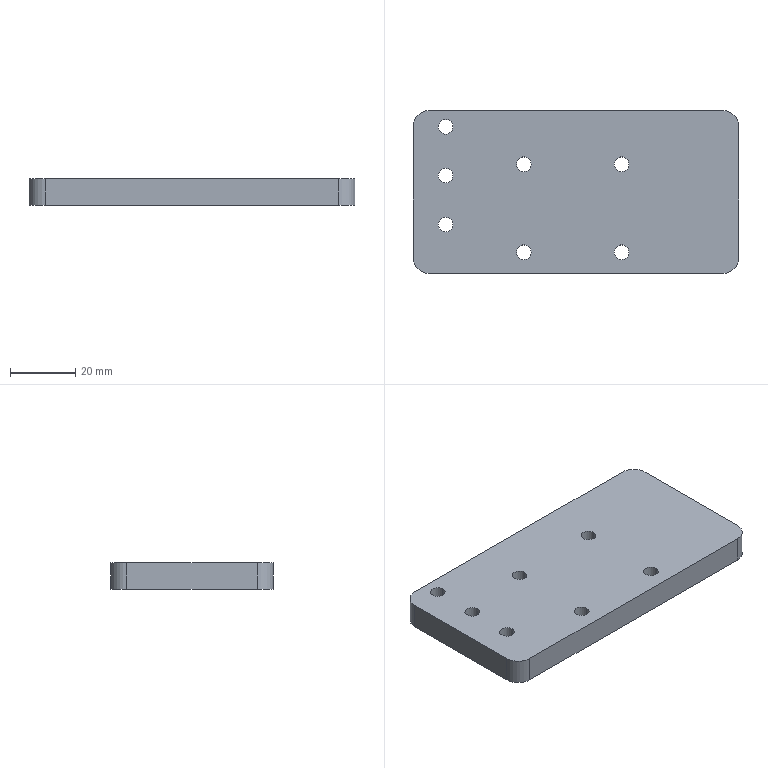Part | STEP file | 08-23 side baffle fixing plate A | 1 solid | 45 faces | box 100 x 50 x 8 mm | volume 37879 mm3 | cylinder 32 | plane 13 | commonest cylinder face diameters 4.5 x14 8 x14 10 x4
STEP:
#1=CARTESIAN_POINT('',(-36.,20.,4.4));
#2=VERTEX_POINT('',#1);
#3=CARTESIAN_POINT('',(-44.,20.,4.4));
#4=VERTEX_POINT('',#3);
#5=CARTESIAN_POINT('',(-40.,20.,4.4));
#6=DIRECTION('',(0.,0.,-1.));
#7=DIRECTION('',(-1.,0.,0.));
#8=AXIS2_PLACEMENT_3D('',#5,#6,#7);
#9=CIRCLE('',#8,4.);
#10=EDGE_CURVE('',#2,#4,#9,.T.);
#11=ORIENTED_EDGE('',*,*,#10,.F.);
#12=CARTESIAN_POINT('',(-36.,20.,0.));
#13=VERTEX_POINT('',#12);
#14=CARTESIAN_POINT('',(-36.,20.,0.));
#15=DIRECTION('',(0.,0.,-1.));
#16=VECTOR('',#15,1000.);
#17=LINE('',#14,#16);
#18=EDGE_CURVE('',#2,#13,#17,.T.);
#19=ORIENTED_EDGE('',*,*,#18,.T.);
#20=CARTESIAN_POINT('',(-44.,20.,0.));
#21=VERTEX_POINT('',#20);
#22=CARTESIAN_POINT('',(-40.,20.,0.));
#23=DIRECTION('',(0.,0.,-1.));
#24=DIRECTION('',(-1.,0.,0.));
#25=AXIS2_PLACEMENT_3D('',#22,#23,#24);
#26=CIRCLE('',#25,4.);
#27=EDGE_CURVE('',#13,#21,#26,.T.);
#28=ORIENTED_EDGE('',*,*,#27,.T.);
#29=CARTESIAN_POINT('',(-44.,20.,0.));
#30=DIRECTION('',(0.,0.,-1.));
#31=VECTOR('',#30,1000.);
#32=LINE('',#29,#31);
#33=EDGE_CURVE('',#4,#21,#32,.T.);
#34=ORIENTED_EDGE('',*,*,#33,.F.);
#35=EDGE_LOOP('',(#11,#19,#28,#34));
#36=FACE_OUTER_BOUND('',#35,.T.);
#37=CARTESIAN_POINT('',(-40.,20.,0.));
#38=DIRECTION('',(0.,0.,-1.));
#39=DIRECTION('',(-1.,0.,0.));
#40=AXIS2_PLACEMENT_3D('',#37,#38,#39);
#41=CYLINDRICAL_SURFACE('',#40,4.);
#42=ADVANCED_FACE('',(#36),#41,.F.);
#43=CARTESIAN_POINT('',(-37.75,20.,8.));
#44=VERTEX_POINT('',#43);
#45=CARTESIAN_POINT('',(-42.25,20.,8.));
#46=VERTEX_POINT('',#45);
#47=CARTESIAN_POINT('',(-40.,20.,8.));
#48=DIRECTION('',(0.,0.,-1.));
#49=DIRECTION('',(-1.,0.,0.));
#50=AXIS2_PLACEMENT_3D('',#47,#48,#49);
#51=CIRCLE('',#50,2.25);
#52=EDGE_CURVE('',#44,#46,#51,.T.);
#53=ORIENTED_EDGE('',*,*,#52,.F.);
#54=CARTESIAN_POINT('',(-37.75,20.,4.4));
#55=VERTEX_POINT('',#54);
#56=CARTESIAN_POINT('',(-37.75,20.,0.));
#57=DIRECTION('',(0.,0.,-1.));
#58=VECTOR('',#57,1000.);
#59=LINE('',#56,#58);
#60=EDGE_CURVE('',#44,#55,#59,.T.);
#61=ORIENTED_EDGE('',*,*,#60,.T.);
#62=CARTESIAN_POINT('',(-42.25,20.,4.4));
#63=VERTEX_POINT('',#62);
#64=CARTESIAN_POINT('',(-40.,20.,4.4));
#65=DIRECTION('',(0.,0.,-1.));
#66=DIRECTION('',(-1.,0.,0.));
#67=AXIS2_PLACEMENT_3D('',#64,#65,#66);
#68=CIRCLE('',#67,2.25);
#69=EDGE_CURVE('',#55,#63,#68,.T.);
#70=ORIENTED_EDGE('',*,*,#69,.T.);
#71=CARTESIAN_POINT('',(-42.25,20.,0.));
#72=DIRECTION('',(0.,0.,-1.));
#73=VECTOR('',#72,1000.);
#74=LINE('',#71,#73);
#75=EDGE_CURVE('',#46,#63,#74,.T.);
#76=ORIENTED_EDGE('',*,*,#75,.F.);
#77=EDGE_LOOP('',(#53,#61,#70,#76));
#78=FACE_OUTER_BOUND('',#77,.T.);
#79=CARTESIAN_POINT('',(-40.,20.,0.));
#80=DIRECTION('',(0.,0.,-1.));
#81=DIRECTION('',(-1.,0.,0.));
#82=AXIS2_PLACEMENT_3D('',#79,#80,#81);
#83=CYLINDRICAL_SURFACE('',#82,2.25);
#84=ADVANCED_FACE('',(#78),#83,.F.);
#85=CARTESIAN_POINT('',(-36.,5.,4.4));
#86=VERTEX_POINT('',#85);
#87=CARTESIAN_POINT('',(-44.,5.,4.4));
#88=VERTEX_POINT('',#87);
#89=CARTESIAN_POINT('',(-40.,5.,4.4));
#90=DIRECTION('',(0.,0.,-1.));
#91=DIRECTION('',(-1.,0.,0.));
#92=AXIS2_PLACEMENT_3D('',#89,#90,#91);
#93=CIRCLE('',#92,4.);
#94=EDGE_CURVE('',#86,#88,#93,.T.);
#95=ORIENTED_EDGE('',*,*,#94,.F.);
#96=CARTESIAN_POINT('',(-36.,5.,0.));
#97=VERTEX_POINT('',#96);
#98=CARTESIAN_POINT('',(-36.,5.,0.));
#99=DIRECTION('',(0.,0.,-1.));
#100=VECTOR('',#99,1000.);
#101=LINE('',#98,#100);
#102=EDGE_CURVE('',#86,#97,#101,.T.);
#103=ORIENTED_EDGE('',*,*,#102,.T.);
#104=CARTESIAN_POINT('',(-44.,5.,0.));
#105=VERTEX_POINT('',#104);
#106=CARTESIAN_POINT('',(-40.,5.,0.));
#107=DIRECTION('',(0.,0.,-1.));
#108=DIRECTION('',(-1.,0.,0.));
#109=AXIS2_PLACEMENT_3D('',#106,#107,#108);
#110=CIRCLE('',#109,4.);
#111=EDGE_CURVE('',#97,#105,#110,.T.);
#112=ORIENTED_EDGE('',*,*,#111,.T.);
#113=CARTESIAN_POINT('',(-44.,5.,0.));
#114=DIRECTION('',(0.,0.,-1.));
#115=VECTOR('',#114,1000.);
#116=LINE('',#113,#115);
#117=EDGE_CURVE('',#88,#105,#116,.T.);
#118=ORIENTED_EDGE('',*,*,#117,.F.);
#119=EDGE_LOOP('',(#95,#103,#112,#118));
#120=FACE_OUTER_BOUND('',#119,.T.);
#121=CARTESIAN_POINT('',(-40.,5.,0.));
#122=DIRECTION('',(0.,0.,-1.));
#123=DIRECTION('',(-1.,0.,0.));
#124=AXIS2_PLACEMENT_3D('',#121,#122,#123);
#125=CYLINDRICAL_SURFACE('',#124,4.);
#126=ADVANCED_FACE('',(#120),#125,.F.);
#127=CARTESIAN_POINT('',(-37.75,5.,8.));
#128=VERTEX_POINT('',#127);
#129=CARTESIAN_POINT('',(-42.25,5.,8.));
#130=VERTEX_POINT('',#129);
#131=CARTESIAN_POINT('',(-40.,5.,8.));
#132=DIRECTION('',(0.,0.,-1.));
#133=DIRECTION('',(-1.,0.,0.));
#134=AXIS2_PLACEMENT_3D('',#131,#132,#133);
#135=CIRCLE('',#134,2.25);
#136=EDGE_CURVE('',#128,#130,#135,.T.);
#137=ORIENTED_EDGE('',*,*,#136,.F.);
#138=CARTESIAN_POINT('',(-37.75,5.,4.4));
#139=VERTEX_POINT('',#138);
#140=CARTESIAN_POINT('',(-37.75,5.,0.));
#141=DIRECTION('',(0.,0.,-1.));
#142=VECTOR('',#141,1000.);
#143=LINE('',#140,#142);
#144=EDGE_CURVE('',#128,#139,#143,.T.);
#145=ORIENTED_EDGE('',*,*,#144,.T.);
#146=CARTESIAN_POINT('',(-42.25,5.,4.4));
#147=VERTEX_POINT('',#146);
#148=CARTESIAN_POINT('',(-40.,5.,4.4));
#149=DIRECTION('',(0.,0.,-1.));
#150=DIRECTION('',(-1.,0.,0.));
#151=AXIS2_PLACEMENT_3D('',#148,#149,#150);
#152=CIRCLE('',#151,2.25);
#153=EDGE_CURVE('',#139,#147,#152,.T.);
#154=ORIENTED_EDGE('',*,*,#153,.T.);
#155=CARTESIAN_POINT('',(-42.25,5.,0.));
#156=DIRECTION('',(0.,0.,-1.));
#157=VECTOR('',#156,1000.);
#158=LINE('',#155,#157);
#159=EDGE_CURVE('',#130,#147,#158,.T.);
#160=ORIENTED_EDGE('',*,*,#159,.F.);
#161=EDGE_LOOP('',(#137,#145,#154,#160));
#162=FACE_OUTER_BOUND('',#161,.T.);
#163=CARTESIAN_POINT('',(-40.,5.,0.));
#164=DIRECTION('',(0.,0.,-1.));
#165=DIRECTION('',(-1.,0.,0.));
#166=AXIS2_PLACEMENT_3D('',#163,#164,#165);
#167=CYLINDRICAL_SURFACE('',#166,2.25);
#168=ADVANCED_FACE('',(#162),#167,.F.);
#169=CARTESIAN_POINT('',(-36.,-10.,4.4));
#170=VERTEX_POINT('',#169);
#171=CARTESIAN_POINT('',(-44.,-10.,4.4));
#172=VERTEX_POINT('',#171);
#173=CARTESIAN_POINT('',(-40.,-10.,4.4));
#174=DIRECTION('',(0.,0.,-1.));
#175=DIRECTION('',(-1.,0.,0.));
#176=AXIS2_PLACEMENT_3D('',#173,#174,#175);
#177=CIRCLE('',#176,4.);
#178=EDGE_CURVE('',#170,#172,#177,.T.);
#179=ORIENTED_EDGE('',*,*,#178,.F.);
#180=CARTESIAN_POINT('',(-36.,-10.,0.));
#181=VERTEX_POINT('',#180);
#182=CARTESIAN_POINT('',(-36.,-10.,0.));
#183=DIRECTION('',(0.,0.,-1.));
#184=VECTOR('',#183,1000.);
#185=LINE('',#182,#184);
#186=EDGE_CURVE('',#170,#181,#185,.T.);
#187=ORIENTED_EDGE('',*,*,#186,.T.);
#188=CARTESIAN_POINT('',(-44.,-10.,0.));
#189=VERTEX_POINT('',#188);
#190=CARTESIAN_POINT('',(-40.,-10.,0.));
#191=DIRECTION('',(0.,0.,-1.));
#192=DIRECTION('',(-1.,0.,0.));
#193=AXIS2_PLACEMENT_3D('',#190,#191,#192);
#194=CIRCLE('',#193,4.);
#195=EDGE_CURVE('',#181,#189,#194,.T.);
#196=ORIENTED_EDGE('',*,*,#195,.T.);
#197=CARTESIAN_POINT('',(-44.,-10.,0.));
#198=DIRECTION('',(0.,0.,-1.));
#199=VECTOR('',#198,1000.);
#200=LINE('',#197,#199);
#201=EDGE_CURVE('',#172,#189,#200,.T.);
#202=ORIENTED_EDGE('',*,*,#201,.F.);
#203=EDGE_LOOP('',(#179,#187,#196,#202));
#204=FACE_OUTER_BOUND('',#203,.T.);
#205=CARTESIAN_POINT('',(-40.,-10.,0.));
#206=DIRECTION('',(0.,0.,-1.));
#207=DIRECTION('',(-1.,0.,0.));
#208=AXIS2_PLACEMENT_3D('',#205,#206,#207);
#209=CYLINDRICAL_SURFACE('',#208,4.);
#210=ADVANCED_FACE('',(#204),#209,.F.);
#211=CARTESIAN_POINT('',(-37.75,-10.,8.));
#212=VERTEX_POINT('',#211);
#213=CARTESIAN_POINT('',(-42.25,-10.,8.));
#214=VERTEX_POINT('',#213);
#215=CARTESIAN_POINT('',(-40.,-10.,8.));
#216=DIRECTION('',(0.,0.,-1.));
#217=DIRECTION('',(-1.,0.,0.));
#218=AXIS2_PLACEMENT_3D('',#215,#216,#217);
#219=CIRCLE('',#218,2.25);
#220=EDGE_CURVE('',#212,#214,#219,.T.);
#221=ORIENTED_EDGE('',*,*,#220,.F.);
#222=CARTESIAN_POINT('',(-37.75,-10.,4.4));
#223=VERTEX_POINT('',#222);
#224=CARTESIAN_POINT('',(-37.75,-10.,0.));
#225=DIRECTION('',(0.,0.,-1.));
#226=VECTOR('',#225,1000.);
#227=LINE('',#224,#226);
#228=EDGE_CURVE('',#212,#223,#227,.T.);
#229=ORIENTED_EDGE('',*,*,#228,.T.);
#230=CARTESIAN_POINT('',(-42.25,-10.,4.4));
#231=VERTEX_POINT('',#230);
#232=CARTESIAN_POINT('',(-40.,-10.,4.4));
#233=DIRECTION('',(0.,0.,-1.));
#234=DIRECTION('',(-1.,0.,0.));
#235=AXIS2_PLACEMENT_3D('',#232,#233,#234);
#236=CIRCLE('',#235,2.25);
#237=EDGE_CURVE('',#223,#231,#236,.T.);
#238=ORIENTED_EDGE('',*,*,#237,.T.);
#239=CARTESIAN_POINT('',(-42.25,-10.,0.));
#240=DIRECTION('',(0.,0.,-1.));
#241=VECTOR('',#240,1000.);
#242=LINE('',#239,#241);
#243=EDGE_CURVE('',#214,#231,#242,.T.);
#244=ORIENTED_EDGE('',*,*,#243,.F.);
#245=EDGE_LOOP('',(#221,#229,#238,#244));
#246=FACE_OUTER_BOUND('',#245,.T.);
#247=CARTESIAN_POINT('',(-40.,-10.,0.));
#248=DIRECTION('',(0.,0.,-1.));
#249=DIRECTION('',(-1.,0.,0.));
#250=AXIS2_PLACEMENT_3D('',#247,#248,#249);
#251=CYLINDRICAL_SURFACE('',#250,2.25);
#252=ADVANCED_FACE('',(#246),#251,.F.);
#253=CARTESIAN_POINT('',(18.,8.5,4.4));
#254=VERTEX_POINT('',#253);
#255=CARTESIAN_POINT('',(10.,8.5,4.4));
#256=VERTEX_POINT('',#255);
#257=CARTESIAN_POINT('',(14.,8.5,4.4));
#258=DIRECTION('',(0.,0.,-1.));
#259=DIRECTION('',(-1.,0.,0.));
#260=AXIS2_PLACEMENT_3D('',#257,#258,#259);
#261=CIRCLE('',#260,4.);
#262=EDGE_CURVE('',#254,#256,#261,.T.);
#263=ORIENTED_EDGE('',*,*,#262,.F.);
#264=CARTESIAN_POINT('',(18.,8.5,0.));
#265=VERTEX_POINT('',#264);
#266=CARTESIAN_POINT('',(18.,8.5,0.));
#267=DIRECTION('',(0.,0.,-1.));
#268=VECTOR('',#267,1000.);
#269=LINE('',#266,#268);
#270=EDGE_CURVE('',#254,#265,#269,.T.);
#271=ORIENTED_EDGE('',*,*,#270,.T.);
#272=CARTESIAN_POINT('',(10.,8.5,0.));
#273=VERTEX_POINT('',#272);
#274=CARTESIAN_POINT('',(14.,8.5,0.));
#275=DIRECTION('',(0.,0.,-1.));
#276=DIRECTION('',(-1.,0.,0.));
#277=AXIS2_PLACEMENT_3D('',#274,#275,#276);
#278=CIRCLE('',#277,4.);
#279=EDGE_CURVE('',#265,#273,#278,.T.);
#280=ORIENTED_EDGE('',*,*,#279,.T.);
#281=CARTESIAN_POINT('',(10.,8.5,0.));
#282=DIRECTION('',(0.,0.,-1.));
#283=VECTOR('',#282,1000.);
#284=LINE('',#281,#283);
#285=EDGE_CURVE('',#256,#273,#284,.T.);
#286=ORIENTED_EDGE('',*,*,#285,.F.);
#287=EDGE_LOOP('',(#263,#271,#280,#286));
#288=FACE_OUTER_BOUND('',#287,.T.);
#289=CARTESIAN_POINT('',(14.,8.5,0.));
#290=DIRECTION('',(0.,0.,-1.));
#291=DIRECTION('',(-1.,0.,0.));
#292=AXIS2_PLACEMENT_3D('',#289,#290,#291);
#293=CYLINDRICAL_SURFACE('',#292,4.);
#294=ADVANCED_FACE('',(#288),#293,.F.);
#295=CARTESIAN_POINT('',(16.25,8.5,8.));
#296=VERTEX_POINT('',#295);
#297=CARTESIAN_POINT('',(11.75,8.5,8.));
#298=VERTEX_POINT('',#297);
#299=CARTESIAN_POINT('',(14.,8.5,8.));
#300=DIRECTION('',(0.,0.,-1.));
#301=DIRECTION('',(-1.,0.,0.));
#302=AXIS2_PLACEMENT_3D('',#299,#300,#301);
#303=CIRCLE('',#302,2.25);
#304=EDGE_CURVE('',#296,#298,#303,.T.);
#305=ORIENTED_EDGE('',*,*,#304,.F.);
#306=CARTESIAN_POINT('',(16.25,8.5,4.4));
#307=VERTEX_POINT('',#306);
#308=CARTESIAN_POINT('',(16.25,8.5,0.));
#309=DIRECTION('',(0.,0.,-1.));
#310=VECTOR('',#309,1000.);
#311=LINE('',#308,#310);
#312=EDGE_CURVE('',#296,#307,#311,.T.);
#313=ORIENTED_EDGE('',*,*,#312,.T.);
#314=CARTESIAN_POINT('',(11.75,8.5,4.4));
#315=VERTEX_POINT('',#314);
#316=CARTESIAN_POINT('',(14.,8.5,4.4));
#317=DIRECTION('',(0.,0.,-1.));
#318=DIRECTION('',(-1.,0.,0.));
#319=AXIS2_PLACEMENT_3D('',#316,#317,#318);
#320=CIRCLE('',#319,2.25);
#321=EDGE_CURVE('',#307,#315,#320,.T.);
#322=ORIENTED_EDGE('',*,*,#321,.T.);
#323=CARTESIAN_POINT('',(11.75,8.5,0.));
#324=DIRECTION('',(0.,0.,-1.));
#325=VECTOR('',#324,1000.);
#326=LINE('',#323,#325);
#327=EDGE_CURVE('',#298,#315,#326,.T.);
#328=ORIENTED_EDGE('',*,*,#327,.F.);
#329=EDGE_LOOP('',(#305,#313,#322,#328));
#330=FACE_OUTER_BOUND('',#329,.T.);
#331=CARTESIAN_POINT('',(14.,8.5,0.));
#332=DIRECTION('',(0.,0.,-1.));
#333=DIRECTION('',(-1.,0.,0.));
#334=AXIS2_PLACEMENT_3D('',#331,#332,#333);
#335=CYLINDRICAL_SURFACE('',#334,2.25);
#336=ADVANCED_FACE('',(#330),#335,.F.);
#337=CARTESIAN_POINT('',(-12.,8.5,4.4));
#338=VERTEX_POINT('',#337);
#339=CARTESIAN_POINT('',(-20.,8.5,4.4));
#340=VERTEX_POINT('',#339);
#341=CARTESIAN_POINT('',(-16.,8.5,4.4));
#342=DIRECTION('',(0.,0.,-1.));
#343=DIRECTION('',(-1.,0.,0.));
#344=AXIS2_PLACEMENT_3D('',#341,#342,#343);
#345=CIRCLE('',#344,4.);
#346=EDGE_CURVE('',#338,#340,#345,.T.);
#347=ORIENTED_EDGE('',*,*,#346,.F.);
#348=CARTESIAN_POINT('',(-12.,8.5,0.));
#349=VERTEX_POINT('',#348);
#350=CARTESIAN_POINT('',(-12.,8.5,0.));
#351=DIRECTION('',(0.,0.,-1.));
#352=VECTOR('',#351,1000.);
#353=LINE('',#350,#352);
#354=EDGE_CURVE('',#338,#349,#353,.T.);
#355=ORIENTED_EDGE('',*,*,#354,.T.);
#356=CARTESIAN_POINT('',(-20.,8.5,0.));
#357=VERTEX_POINT('',#356);
#358=CARTESIAN_POINT('',(-16.,8.5,0.));
#359=DIRECTION('',(0.,0.,-1.));
#360=DIRECTION('',(-1.,0.,0.));
#361=AXIS2_PLACEMENT_3D('',#358,#359,#360);
#362=CIRCLE('',#361,4.);
#363=EDGE_CURVE('',#349,#357,#362,.T.);
#364=ORIENTED_EDGE('',*,*,#363,.T.);
#365=CARTESIAN_POINT('',(-20.,8.5,0.));
#366=DIRECTION('',(0.,0.,-1.));
#367=VECTOR('',#366,1000.);
#368=LINE('',#365,#367);
#369=EDGE_CURVE('',#340,#357,#368,.T.);
#370=ORIENTED_EDGE('',*,*,#369,.F.);
#371=EDGE_LOOP('',(#347,#355,#364,#370));
#372=FACE_OUTER_BOUND('',#371,.T.);
#373=CARTESIAN_POINT('',(-16.,8.5,0.));
#374=DIRECTION('',(0.,0.,-1.));
#375=DIRECTION('',(-1.,0.,0.));
#376=AXIS2_PLACEMENT_3D('',#373,#374,#375);
#377=CYLINDRICAL_SURFACE('',#376,4.);
#378=ADVANCED_FACE('',(#372),#377,.F.);
#379=CARTESIAN_POINT('',(-13.75,8.5,8.));
#380=VERTEX_POINT('',#379);
#381=CARTESIAN_POINT('',(-18.25,8.5,8.));
#382=VERTEX_POINT('',#381);
#383=CARTESIAN_POINT('',(-16.,8.5,8.));
#384=DIRECTION('',(0.,0.,-1.));
#385=DIRECTION('',(-1.,0.,0.));
#386=AXIS2_PLACEMENT_3D('',#383,#384,#385);
#387=CIRCLE('',#386,2.25);
#388=EDGE_CURVE('',#380,#382,#387,.T.);
#389=ORIENTED_EDGE('',*,*,#388,.F.);
#390=CARTESIAN_POINT('',(-13.75,8.5,4.4));
#391=VERTEX_POINT('',#390);
#392=CARTESIAN_POINT('',(-13.75,8.5,0.));
#393=DIRECTION('',(0.,0.,-1.));
#394=VECTOR('',#393,1000.);
#395=LINE('',#392,#394);
#396=EDGE_CURVE('',#380,#391,#395,.T.);
#397=ORIENTED_EDGE('',*,*,#396,.T.);
#398=CARTESIAN_POINT('',(-18.25,8.5,4.4));
#399=VERTEX_POINT('',#398);
#400=CARTESIAN_POINT('',(-16.,8.5,4.4));
#401=DIRECTION('',(0.,0.,-1.));
#402=DIRECTION('',(-1.,0.,0.));
#403=AXIS2_PLACEMENT_3D('',#400,#401,#402);
#404=CIRCLE('',#403,2.25);
#405=EDGE_CURVE('',#391,#399,#404,.T.);
#406=ORIENTED_EDGE('',*,*,#405,.T.);
#407=CARTESIAN_POINT('',(-18.25,8.5,0.));
#408=DIRECTION('',(0.,0.,-1.));
#409=VECTOR('',#408,1000.);
#410=LINE('',#407,#409);
#411=EDGE_CURVE('',#382,#399,#410,.T.);
#412=ORIENTED_EDGE('',*,*,#411,.F.);
#413=EDGE_LOOP('',(#389,#397,#406,#412));
#414=FACE_OUTER_BOUND('',#413,.T.);
#415=CARTESIAN_POINT('',(-16.,8.5,0.));
#416=DIRECTION('',(0.,0.,-1.));
#417=DIRECTION('',(-1.,0.,0.));
#418=AXIS2_PLACEMENT_3D('',#415,#416,#417);
#419=CYLINDRICAL_SURFACE('',#418,2.25);
#420=ADVANCED_FACE('',(#414),#419,.F.);
#421=CARTESIAN_POINT('',(-12.,-18.5,4.4));
#422=VERTEX_POINT('',#421);
#423=CARTESIAN_POINT('',(-20.,-18.5,4.4));
#424=VERTEX_POINT('',#423);
#425=CARTESIAN_POINT('',(-16.,-18.5,4.4));
#426=DIRECTION('',(0.,0.,-1.));
#427=DIRECTION('',(-1.,0.,0.));
#428=AXIS2_PLACEMENT_3D('',#425,#426,#427);
#429=CIRCLE('',#428,4.);
#430=EDGE_CURVE('',#422,#424,#429,.T.);
#431=ORIENTED_EDGE('',*,*,#430,.F.);
#432=CARTESIAN_POINT('',(-12.,-18.5,0.));
#433=VERTEX_POINT('',#432);
#434=CARTESIAN_POINT('',(-12.,-18.5,0.));
#435=DIRECTION('',(0.,0.,-1.));
#436=VECTOR('',#435,1000.);
#437=LINE('',#434,#436);
#438=EDGE_CURVE('',#422,#433,#437,.T.);
#439=ORIENTED_EDGE('',*,*,#438,.T.);
#440=CARTESIAN_POINT('',(-20.,-18.5,0.));
#441=VERTEX_POINT('',#440);
#442=CARTESIAN_POINT('',(-16.,-18.5,0.));
#443=DIRECTION('',(0.,0.,-1.));
#444=DIRECTION('',(-1.,0.,0.));
#445=AXIS2_PLACEMENT_3D('',#442,#443,#444);
#446=CIRCLE('',#445,4.);
#447=EDGE_CURVE('',#433,#441,#446,.T.);
#448=ORIENTED_EDGE('',*,*,#447,.T.);
#449=CARTESIAN_POINT('',(-20.,-18.5,0.));
#450=DIRECTION('',(0.,0.,-1.));
#451=VECTOR('',#450,1000.);
#452=LINE('',#449,#451);
#453=EDGE_CURVE('',#424,#441,#452,.T.);
#454=ORIENTED_EDGE('',*,*,#453,.F.);
#455=EDGE_LOOP('',(#431,#439,#448,#454));
#456=FACE_OUTER_BOUND('',#455,.T.);
#457=CARTESIAN_POINT('',(-16.,-18.5,0.));
#458=DIRECTION('',(0.,0.,-1.));
#459=DIRECTION('',(-1.,0.,0.));
#460=AXIS2_PLACEMENT_3D('',#457,#458,#459);
#461=CYLINDRICAL_SURFACE('',#460,4.);
#462=ADVANCED_FACE('',(#456),#461,.F.);
#463=CARTESIAN_POINT('',(-13.75,-18.5,8.));
#464=VERTEX_POINT('',#463);
#465=CARTESIAN_POINT('',(-18.25,-18.5,8.));
#466=VERTEX_POINT('',#465);
#467=CARTESIAN_POINT('',(-16.,-18.5,8.));
#468=DIRECTION('',(0.,0.,-1.));
#469=DIRECTION('',(-1.,0.,0.));
#470=AXIS2_PLACEMENT_3D('',#467,#468,#469);
#471=CIRCLE('',#470,2.25);
#472=EDGE_CURVE('',#464,#466,#471,.T.);
#473=ORIENTED_EDGE('',*,*,#472,.F.);
#474=CARTESIAN_POINT('',(-13.75,-18.5,4.4));
#475=VERTEX_POINT('',#474);
#476=CARTESIAN_POINT('',(-13.75,-18.5,0.));
#477=DIRECTION('',(0.,0.,-1.));
#478=VECTOR('',#477,1000.);
#479=LINE('',#476,#478);
#480=EDGE_CURVE('',#464,#475,#479,.T.);
#481=ORIENTED_EDGE('',*,*,#480,.T.);
#482=CARTESIAN_POINT('',(-18.25,-18.5,4.4));
#483=VERTEX_POINT('',#482);
#484=CARTESIAN_POINT('',(-16.,-18.5,4.4));
#485=DIRECTION('',(0.,0.,-1.));
#486=DIRECTION('',(-1.,0.,0.));
#487=AXIS2_PLACEMENT_3D('',#484,#485,#486);
#488=CIRCLE('',#487,2.25);
#489=EDGE_CURVE('',#475,#483,#488,.T.);
#490=ORIENTED_EDGE('',*,*,#489,.T.);
#491=CARTESIAN_POINT('',(-18.25,-18.5,0.));
#492=DIRECTION('',(0.,0.,-1.));
#493=VECTOR('',#492,1000.);
#494=LINE('',#491,#493);
#495=EDGE_CURVE('',#466,#483,#494,.T.);
#496=ORIENTED_EDGE('',*,*,#495,.F.);
#497=EDGE_LOOP('',(#473,#481,#490,#496));
#498=FACE_OUTER_BOUND('',#497,.T.);
#499=CARTESIAN_POINT('',(-16.,-18.5,0.));
#500=DIRECTION('',(0.,0.,-1.));
#501=DIRECTION('',(-1.,0.,0.));
#502=AXIS2_PLACEMENT_3D('',#499,#500,#501);
#503=CYLINDRICAL_SURFACE('',#502,2.25);
#504=ADVANCED_FACE('',(#498),#503,.F.);
#505=CARTESIAN_POINT('',(18.,-18.5,4.4));
#506=VERTEX_POINT('',#505);
#507=CARTESIAN_POINT('',(10.,-18.5,4.4));
#508=VERTEX_POINT('',#507);
#509=CARTESIAN_POINT('',(14.,-18.5,4.4));
#510=DIRECTION('',(0.,0.,-1.));
#511=DIRECTION('',(-1.,0.,0.));
#512=AXIS2_PLACEMENT_3D('',#509,#510,#511);
#513=CIRCLE('',#512,4.);
#514=EDGE_CURVE('',#506,#508,#513,.T.);
#515=ORIENTED_EDGE('',*,*,#514,.F.);
#516=CARTESIAN_POINT('',(18.,-18.5,0.));
#517=VERTEX_POINT('',#516);
#518=CARTESIAN_POINT('',(18.,-18.5,0.));
#519=DIRECTION('',(0.,0.,-1.));
#520=VECTOR('',#519,1000.);
#521=LINE('',#518,#520);
#522=EDGE_CURVE('',#506,#517,#521,.T.);
#523=ORIENTED_EDGE('',*,*,#522,.T.);
#524=CARTESIAN_POINT('',(10.,-18.5,0.));
#525=VERTEX_POINT('',#524);
#526=CARTESIAN_POINT('',(14.,-18.5,0.));
#527=DIRECTION('',(0.,0.,-1.));
#528=DIRECTION('',(-1.,0.,0.));
#529=AXIS2_PLACEMENT_3D('',#526,#527,#528);
#530=CIRCLE('',#529,4.);
#531=EDGE_CURVE('',#517,#525,#530,.T.);
#532=ORIENTED_EDGE('',*,*,#531,.T.);
#533=CARTESIAN_POINT('',(10.,-18.5,0.));
#534=DIRECTION('',(0.,0.,-1.));
#535=VECTOR('',#534,1000.);
#536=LINE('',#533,#535);
#537=EDGE_CURVE('',#508,#525,#536,.T.);
#538=ORIENTED_EDGE('',*,*,#537,.F.);
#539=EDGE_LOOP('',(#515,#523,#532,#538));
#540=FACE_OUTER_BOUND('',#539,.T.);
#541=CARTESIAN_POINT('',(14.,-18.5,0.));
#542=DIRECTION('',(0.,0.,-1.));
#543=DIRECTION('',(-1.,0.,0.));
#544=AXIS2_PLACEMENT_3D('',#541,#542,#543);
#545=CYLINDRICAL_SURFACE('',#544,4.);
#546=ADVANCED_FACE('',(#540),#545,.F.);
#547=CARTESIAN_POINT('',(16.25,-18.5,8.));
#548=VERTEX_POINT('',#547);
#549=CARTESIAN_POINT('',(11.75,-18.5,8.));
#550=VERTEX_POINT('',#549);
#551=CARTESIAN_POINT('',(14.,-18.5,8.));
#552=DIRECTION('',(0.,0.,-1.));
#553=DIRECTION('',(-1.,0.,0.));
#554=AXIS2_PLACEMENT_3D('',#551,#552,#553);
#555=CIRCLE('',#554,2.25);
#556=EDGE_CURVE('',#548,#550,#555,.T.);
#557=ORIENTED_EDGE('',*,*,#556,.F.);
#558=CARTESIAN_POINT('',(16.25,-18.5,4.4));
#559=VERTEX_POINT('',#558);
#560=CARTESIAN_POINT('',(16.25,-18.5,0.));
#561=DIRECTION('',(0.,0.,-1.));
#562=VECTOR('',#561,1000.);
#563=LINE('',#560,#562);
#564=EDGE_CURVE('',#548,#559,#563,.T.);
#565=ORIENTED_EDGE('',*,*,#564,.T.);
#566=CARTESIAN_POINT('',(11.75,-18.5,4.4));
#567=VERTEX_POINT('',#566);
#568=CARTESIAN_POINT('',(14.,-18.5,4.4));
#569=DIRECTION('',(0.,0.,-1.));
#570=DIRECTION('',(-1.,0.,0.));
#571=AXIS2_PLACEMENT_3D('',#568,#569,#570);
#572=CIRCLE('',#571,2.25);
#573=EDGE_CURVE('',#559,#567,#572,.T.);
#574=ORIENTED_EDGE('',*,*,#573,.T.);
#575=CARTESIAN_POINT('',(11.75,-18.5,0.));
#576=DIRECTION('',(0.,0.,-1.));
#577=VECTOR('',#576,1000.);
#578=LINE('',#575,#577);
#579=EDGE_CURVE('',#550,#567,#578,.T.);
#580=ORIENTED_EDGE('',*,*,#579,.F.);
#581=EDGE_LOOP('',(#557,#565,#574,#580));
#582=FACE_OUTER_BOUND('',#581,.T.);
#583=CARTESIAN_POINT('',(14.,-18.5,0.));
#584=DIRECTION('',(0.,0.,-1.));
#585=DIRECTION('',(-1.,0.,0.));
#586=AXIS2_PLACEMENT_3D('',#583,#584,#585);
#587=CYLINDRICAL_SURFACE('',#586,2.25);
#588=ADVANCED_FACE('',(#582),#587,.F.);
#589=CARTESIAN_POINT('',(50.,-20.,0.));
#590=VERTEX_POINT('',#589);
#591=CARTESIAN_POINT('',(50.,20.,0.));
#592=VERTEX_POINT('',#591);
#593=CARTESIAN_POINT('',(50.,25.,0.));
#594=DIRECTION('',(0.,1.,0.));
#595=VECTOR('',#594,1000.);
#596=LINE('',#593,#595);
#597=EDGE_CURVE('',#590,#592,#596,.T.);
#598=ORIENTED_EDGE('',*,*,#597,.T.);
#599=CARTESIAN_POINT('',(50.,20.,8.));
#600=VERTEX_POINT('',#599);
#601=CARTESIAN_POINT('',(50.,20.,8.));
#602=DIRECTION('',(0.,0.,1.));
#603=VECTOR('',#602,1000.);
#604=LINE('',#601,#603);
#605=EDGE_CURVE('',#592,#600,#604,.T.);
#606=ORIENTED_EDGE('',*,*,#605,.T.);
#607=CARTESIAN_POINT('',(50.,-20.,8.));
#608=VERTEX_POINT('',#607);
#609=CARTESIAN_POINT('',(50.,25.,8.));
#610=DIRECTION('',(0.,1.,0.));
#611=VECTOR('',#610,1000.);
#612=LINE('',#609,#611);
#613=EDGE_CURVE('',#608,#600,#612,.T.);
#614=ORIENTED_EDGE('',*,*,#613,.F.);
#615=CARTESIAN_POINT('',(50.,-20.,8.));
#616=DIRECTION('',(0.,0.,-1.));
#617=VECTOR('',#616,1000.);
#618=LINE('',#615,#617);
#619=EDGE_CURVE('',#608,#590,#618,.T.);
#620=ORIENTED_EDGE('',*,*,#619,.T.);
#621=EDGE_LOOP('',(#598,#606,#614,#620));
#622=FACE_OUTER_BOUND('',#621,.T.);
#623=CARTESIAN_POINT('',(50.,25.,8.));
#624=DIRECTION('',(-1.,0.,0.));
#625=DIRECTION('',(0.,0.,1.));
#626=AXIS2_PLACEMENT_3D('',#623,#624,#625);
#627=PLANE('',#626);
#628=ADVANCED_FACE('',(#622),#627,.F.);
#629=CARTESIAN_POINT('',(45.,25.,8.));
#630=VERTEX_POINT('',#629);
#631=CARTESIAN_POINT('',(-45.,25.,8.));
#632=VERTEX_POINT('',#631);
#633=CARTESIAN_POINT('',(-50.,25.,8.));
#634=DIRECTION('',(-1.,0.,0.));
#635=VECTOR('',#634,1000.);
#636=LINE('',#633,#635);
#637=EDGE_CURVE('',#630,#632,#636,.T.);
#638=ORIENTED_EDGE('',*,*,#637,.F.);
#639=CARTESIAN_POINT('',(45.,25.,0.));
#640=VERTEX_POINT('',#639);
#641=CARTESIAN_POINT('',(45.,25.,8.));
#642=DIRECTION('',(0.,0.,-1.));
#643=VECTOR('',#642,1000.);
#644=LINE('',#641,#643);
#645=EDGE_CURVE('',#630,#640,#644,.T.);
#646=ORIENTED_EDGE('',*,*,#645,.T.);
#647=CARTESIAN_POINT('',(-45.,25.,0.));
#648=VERTEX_POINT('',#647);
#649=CARTESIAN_POINT('',(-50.,25.,0.));
#650=DIRECTION('',(-1.,0.,0.));
#651=VECTOR('',#650,1000.);
#652=LINE('',#649,#651);
#653=EDGE_CURVE('',#640,#648,#652,.T.);
#654=ORIENTED_EDGE('',*,*,#653,.T.);
#655=CARTESIAN_POINT('',(-45.,25.,8.));
#656=DIRECTION('',(0.,0.,1.));
#657=VECTOR('',#656,1000.);
#658=LINE('',#655,#657);
#659=EDGE_CURVE('',#648,#632,#658,.T.);
#660=ORIENTED_EDGE('',*,*,#659,.T.);
#661=EDGE_LOOP('',(#638,#646,#654,#660));
#662=FACE_OUTER_BOUND('',#661,.T.);
#663=CARTESIAN_POINT('',(-50.,25.,8.));
#664=DIRECTION('',(0.,-1.,0.));
#665=DIRECTION('',(0.,0.,-1.));
#666=AXIS2_PLACEMENT_3D('',#663,#664,#665);
#667=PLANE('',#666);
#668=ADVANCED_FACE('',(#662),#667,.F.);
#669=CARTESIAN_POINT('',(-50.,20.,0.));
#670=VERTEX_POINT('',#669);
#671=CARTESIAN_POINT('',(-50.,-20.,0.));
#672=VERTEX_POINT('',#671);
#673=CARTESIAN_POINT('',(-50.,25.,0.));
#674=DIRECTION('',(0.,-1.,0.));
#675=VECTOR('',#674,1000.);
#676=LINE('',#673,#675);
#677=EDGE_CURVE('',#670,#672,#676,.T.);
#678=ORIENTED_EDGE('',*,*,#677,.T.);
#679=CARTESIAN_POINT('',(-50.,-20.,8.));
#680=VERTEX_POINT('',#679);
#681=CARTESIAN_POINT('',(-50.,-20.,8.));
#682=DIRECTION('',(0.,0.,1.));
#683=VECTOR('',#682,1000.);
#684=LINE('',#681,#683);
#685=EDGE_CURVE('',#672,#680,#684,.T.);
#686=ORIENTED_EDGE('',*,*,#685,.T.);
#687=CARTESIAN_POINT('',(-50.,20.,8.));
#688=VERTEX_POINT('',#687);
#689=CARTESIAN_POINT('',(-50.,25.,8.));
#690=DIRECTION('',(0.,-1.,0.));
#691=VECTOR('',#690,1000.);
#692=LINE('',#689,#691);
#693=EDGE_CURVE('',#688,#680,#692,.T.);
#694=ORIENTED_EDGE('',*,*,#693,.F.);
#695=CARTESIAN_POINT('',(-50.,20.,8.));
#696=DIRECTION('',(0.,0.,-1.));
#697=VECTOR('',#696,1000.);
#698=LINE('',#695,#697);
#699=EDGE_CURVE('',#688,#670,#698,.T.);
#700=ORIENTED_EDGE('',*,*,#699,.T.);
#701=EDGE_LOOP('',(#678,#686,#694,#700));
#702=FACE_OUTER_BOUND('',#701,.T.);
#703=CARTESIAN_POINT('',(-50.,25.,8.));
#704=DIRECTION('',(1.,0.,0.));
#705=DIRECTION('',(0.,1.,0.));
#706=AXIS2_PLACEMENT_3D('',#703,#704,#705);
#707=PLANE('',#706);
#708=ADVANCED_FACE('',(#702),#707,.F.);
#709=CARTESIAN_POINT('',(-45.,-25.,0.));
#710=VERTEX_POINT('',#709);
#711=CARTESIAN_POINT('',(45.,-25.,0.));
#712=VERTEX_POINT('',#711);
#713=CARTESIAN_POINT('',(-50.,-25.,0.));
#714=DIRECTION('',(1.,0.,0.));
#715=VECTOR('',#714,1000.);
#716=LINE('',#713,#715);
#717=EDGE_CURVE('',#710,#712,#716,.T.);
#718=ORIENTED_EDGE('',*,*,#717,.T.);
#719=CARTESIAN_POINT('',(45.,-25.,8.));
#720=VERTEX_POINT('',#719);
#721=CARTESIAN_POINT('',(45.,-25.,8.));
#722=DIRECTION('',(0.,0.,1.));
#723=VECTOR('',#722,1000.);
#724=LINE('',#721,#723);
#725=EDGE_CURVE('',#712,#720,#724,.T.);
#726=ORIENTED_EDGE('',*,*,#725,.T.);
#727=CARTESIAN_POINT('',(-45.,-25.,8.));
#728=VERTEX_POINT('',#727);
#729=CARTESIAN_POINT('',(-50.,-25.,8.));
#730=DIRECTION('',(1.,0.,0.));
#731=VECTOR('',#730,1000.);
#732=LINE('',#729,#731);
#733=EDGE_CURVE('',#728,#720,#732,.T.);
#734=ORIENTED_EDGE('',*,*,#733,.F.);
#735=CARTESIAN_POINT('',(-45.,-25.,8.));
#736=DIRECTION('',(0.,0.,-1.));
#737=VECTOR('',#736,1000.);
#738=LINE('',#735,#737);
#739=EDGE_CURVE('',#728,#710,#738,.T.);
#740=ORIENTED_EDGE('',*,*,#739,.T.);
#741=EDGE_LOOP('',(#718,#726,#734,#740));
#742=FACE_OUTER_BOUND('',#741,.T.);
#743=CARTESIAN_POINT('',(-50.,-25.,8.));
#744=DIRECTION('',(0.,1.,0.));
#745=DIRECTION('',(0.,0.,1.));
#746=AXIS2_PLACEMENT_3D('',#743,#744,#745);
#747=PLANE('',#746);
#748=ADVANCED_FACE('',(#742),#747,.F.);
#749=CARTESIAN_POINT('',(-40.,20.,8.));
#750=DIRECTION('',(0.,0.,-1.));
#751=DIRECTION('',(-1.,0.,0.));
#752=AXIS2_PLACEMENT_3D('',#749,#750,#751);
#753=CIRCLE('',#752,2.25);
#754=EDGE_CURVE('',#46,#44,#753,.T.);
#755=ORIENTED_EDGE('',*,*,#754,.T.);
#756=ORIENTED_EDGE('',*,*,#52,.T.);
#757=EDGE_LOOP('',(#755,#756));
#758=FACE_BOUND('',#757,.T.);
#759=CARTESIAN_POINT('',(-40.,5.,8.));
#760=DIRECTION('',(0.,0.,-1.));
#761=DIRECTION('',(-1.,0.,0.));
#762=AXIS2_PLACEMENT_3D('',#759,#760,#761);
#763=CIRCLE('',#762,2.25);
#764=EDGE_CURVE('',#130,#128,#763,.T.);
#765=ORIENTED_EDGE('',*,*,#764,.T.);
#766=ORIENTED_EDGE('',*,*,#136,.T.);
#767=EDGE_LOOP('',(#765,#766));
#768=FACE_BOUND('',#767,.T.);
#769=CARTESIAN_POINT('',(-40.,-10.,8.));
#770=DIRECTION('',(0.,0.,-1.));
#771=DIRECTION('',(-1.,0.,0.));
#772=AXIS2_PLACEMENT_3D('',#769,#770,#771);
#773=CIRCLE('',#772,2.25);
#774=EDGE_CURVE('',#214,#212,#773,.T.);
#775=ORIENTED_EDGE('',*,*,#774,.T.);
#776=ORIENTED_EDGE('',*,*,#220,.T.);
#777=EDGE_LOOP('',(#775,#776));
#778=FACE_BOUND('',#777,.T.);
#779=CARTESIAN_POINT('',(14.,8.5,8.));
#780=DIRECTION('',(0.,0.,-1.));
#781=DIRECTION('',(-1.,0.,0.));
#782=AXIS2_PLACEMENT_3D('',#779,#780,#781);
#783=CIRCLE('',#782,2.25);
#784=EDGE_CURVE('',#298,#296,#783,.T.);
#785=ORIENTED_EDGE('',*,*,#784,.T.);
#786=ORIENTED_EDGE('',*,*,#304,.T.);
#787=EDGE_LOOP('',(#785,#786));
#788=FACE_BOUND('',#787,.T.);
#789=CARTESIAN_POINT('',(-16.,8.5,8.));
#790=DIRECTION('',(0.,0.,-1.));
#791=DIRECTION('',(-1.,0.,0.));
#792=AXIS2_PLACEMENT_3D('',#789,#790,#791);
#793=CIRCLE('',#792,2.25);
#794=EDGE_CURVE('',#382,#380,#793,.T.);
#795=ORIENTED_EDGE('',*,*,#794,.T.);
#796=ORIENTED_EDGE('',*,*,#388,.T.);
#797=EDGE_LOOP('',(#795,#796));
#798=FACE_BOUND('',#797,.T.);
#799=CARTESIAN_POINT('',(-16.,-18.5,8.));
#800=DIRECTION('',(0.,0.,-1.));
#801=DIRECTION('',(-1.,0.,0.));
#802=AXIS2_PLACEMENT_3D('',#799,#800,#801);
#803=CIRCLE('',#802,2.25);
#804=EDGE_CURVE('',#466,#464,#803,.T.);
#805=ORIENTED_EDGE('',*,*,#804,.T.);
#806=ORIENTED_EDGE('',*,*,#472,.T.);
#807=EDGE_LOOP('',(#805,#806));
#808=FACE_BOUND('',#807,.T.);
#809=CARTESIAN_POINT('',(14.,-18.5,8.));
#810=DIRECTION('',(0.,0.,-1.));
#811=DIRECTION('',(-1.,0.,0.));
#812=AXIS2_PLACEMENT_3D('',#809,#810,#811);
#813=CIRCLE('',#812,2.25);
#814=EDGE_CURVE('',#550,#548,#813,.T.);
#815=ORIENTED_EDGE('',*,*,#814,.T.);
#816=ORIENTED_EDGE('',*,*,#556,.T.);
#817=EDGE_LOOP('',(#815,#816));
#818=FACE_BOUND('',#817,.T.);
#819=ORIENTED_EDGE('',*,*,#613,.T.);
#820=CARTESIAN_POINT('',(45.,20.,8.));
#821=DIRECTION('',(0.,0.,1.));
#822=DIRECTION('',(1.,0.,0.));
#823=AXIS2_PLACEMENT_3D('',#820,#821,#822);
#824=CIRCLE('',#823,5.);
#825=EDGE_CURVE('',#600,#630,#824,.T.);
#826=ORIENTED_EDGE('',*,*,#825,.T.);
#827=ORIENTED_EDGE('',*,*,#637,.T.);
#828=CARTESIAN_POINT('',(-45.,20.,8.));
#829=DIRECTION('',(0.,0.,1.));
#830=DIRECTION('',(1.,0.,0.));
#831=AXIS2_PLACEMENT_3D('',#828,#829,#830);
#832=CIRCLE('',#831,5.);
#833=EDGE_CURVE('',#632,#688,#832,.T.);
#834=ORIENTED_EDGE('',*,*,#833,.T.);
#835=ORIENTED_EDGE('',*,*,#693,.T.);
#836=CARTESIAN_POINT('',(-45.,-20.,8.));
#837=DIRECTION('',(0.,0.,1.));
#838=DIRECTION('',(1.,0.,0.));
#839=AXIS2_PLACEMENT_3D('',#836,#837,#838);
#840=CIRCLE('',#839,5.);
#841=EDGE_CURVE('',#680,#728,#840,.T.);
#842=ORIENTED_EDGE('',*,*,#841,.T.);
#843=ORIENTED_EDGE('',*,*,#733,.T.);
#844=CARTESIAN_POINT('',(45.,-20.,8.));
#845=DIRECTION('',(0.,0.,1.));
#846=DIRECTION('',(1.,0.,0.));
#847=AXIS2_PLACEMENT_3D('',#844,#845,#846);
#848=CIRCLE('',#847,5.);
#849=EDGE_CURVE('',#720,#608,#848,.T.);
#850=ORIENTED_EDGE('',*,*,#849,.T.);
#851=EDGE_LOOP('',(#819,#826,#827,#834,#835,#842,#843,#850));
#852=FACE_OUTER_BOUND('',#851,.T.);
#853=CARTESIAN_POINT('',(50.,-25.,8.));
#854=DIRECTION('',(0.,0.,1.));
#855=DIRECTION('',(1.,0.,0.));
#856=AXIS2_PLACEMENT_3D('',#853,#854,#855);
#857=PLANE('',#856);
#858=ADVANCED_FACE('',(#758,#768,#778,#788,#798,#808,#818,#852),#857,.T.);
#859=CARTESIAN_POINT('',(-40.,20.,0.));
#860=DIRECTION('',(0.,0.,-1.));
#861=DIRECTION('',(-1.,0.,0.));
#862=AXIS2_PLACEMENT_3D('',#859,#860,#861);
#863=CIRCLE('',#862,4.);
#864=EDGE_CURVE('',#21,#13,#863,.T.);
#865=ORIENTED_EDGE('',*,*,#864,.F.);
#866=ORIENTED_EDGE('',*,*,#27,.F.);
#867=EDGE_LOOP('',(#865,#866));
#868=FACE_BOUND('',#867,.T.);
#869=CARTESIAN_POINT('',(-40.,5.,0.));
#870=DIRECTION('',(0.,0.,-1.));
#871=DIRECTION('',(-1.,0.,0.));
#872=AXIS2_PLACEMENT_3D('',#869,#870,#871);
#873=CIRCLE('',#872,4.);
#874=EDGE_CURVE('',#105,#97,#873,.T.);
#875=ORIENTED_EDGE('',*,*,#874,.F.);
#876=ORIENTED_EDGE('',*,*,#111,.F.);
#877=EDGE_LOOP('',(#875,#876));
#878=FACE_BOUND('',#877,.T.);
#879=CARTESIAN_POINT('',(-40.,-10.,0.));
#880=DIRECTION('',(0.,0.,-1.));
#881=DIRECTION('',(-1.,0.,0.));
#882=AXIS2_PLACEMENT_3D('',#879,#880,#881);
#883=CIRCLE('',#882,4.);
#884=EDGE_CURVE('',#189,#181,#883,.T.);
#885=ORIENTED_EDGE('',*,*,#884,.F.);
#886=ORIENTED_EDGE('',*,*,#195,.F.);
#887=EDGE_LOOP('',(#885,#886));
#888=FACE_BOUND('',#887,.T.);
#889=CARTESIAN_POINT('',(14.,8.5,0.));
#890=DIRECTION('',(0.,0.,-1.));
#891=DIRECTION('',(-1.,0.,0.));
#892=AXIS2_PLACEMENT_3D('',#889,#890,#891);
#893=CIRCLE('',#892,4.);
#894=EDGE_CURVE('',#273,#265,#893,.T.);
#895=ORIENTED_EDGE('',*,*,#894,.F.);
#896=ORIENTED_EDGE('',*,*,#279,.F.);
#897=EDGE_LOOP('',(#895,#896));
#898=FACE_BOUND('',#897,.T.);
#899=CARTESIAN_POINT('',(-16.,8.5,0.));
#900=DIRECTION('',(0.,0.,-1.));
#901=DIRECTION('',(-1.,0.,0.));
#902=AXIS2_PLACEMENT_3D('',#899,#900,#901);
#903=CIRCLE('',#902,4.);
#904=EDGE_CURVE('',#357,#349,#903,.T.);
#905=ORIENTED_EDGE('',*,*,#904,.F.);
#906=ORIENTED_EDGE('',*,*,#363,.F.);
#907=EDGE_LOOP('',(#905,#906));
#908=FACE_BOUND('',#907,.T.);
#909=CARTESIAN_POINT('',(-16.,-18.5,0.));
#910=DIRECTION('',(0.,0.,-1.));
#911=DIRECTION('',(-1.,0.,0.));
#912=AXIS2_PLACEMENT_3D('',#909,#910,#911);
#913=CIRCLE('',#912,4.);
#914=EDGE_CURVE('',#441,#433,#913,.T.);
#915=ORIENTED_EDGE('',*,*,#914,.F.);
#916=ORIENTED_EDGE('',*,*,#447,.F.);
#917=EDGE_LOOP('',(#915,#916));
#918=FACE_BOUND('',#917,.T.);
#919=CARTESIAN_POINT('',(14.,-18.5,0.));
#920=DIRECTION('',(0.,0.,-1.));
#921=DIRECTION('',(-1.,0.,0.));
#922=AXIS2_PLACEMENT_3D('',#919,#920,#921);
#923=CIRCLE('',#922,4.);
#924=EDGE_CURVE('',#525,#517,#923,.T.);
#925=ORIENTED_EDGE('',*,*,#924,.F.);
#926=ORIENTED_EDGE('',*,*,#531,.F.);
#927=EDGE_LOOP('',(#925,#926));
#928=FACE_BOUND('',#927,.T.);
#929=ORIENTED_EDGE('',*,*,#653,.F.);
#930=CARTESIAN_POINT('',(45.,20.,0.));
#931=DIRECTION('',(0.,0.,-1.));
#932=DIRECTION('',(1.,0.,0.));
#933=AXIS2_PLACEMENT_3D('',#930,#931,#932);
#934=CIRCLE('',#933,5.);
#935=EDGE_CURVE('',#640,#592,#934,.T.);
#936=ORIENTED_EDGE('',*,*,#935,.T.);
#937=ORIENTED_EDGE('',*,*,#597,.F.);
#938=CARTESIAN_POINT('',(45.,-20.,0.));
#939=DIRECTION('',(0.,0.,-1.));
#940=DIRECTION('',(1.,0.,0.));
#941=AXIS2_PLACEMENT_3D('',#938,#939,#940);
#942=CIRCLE('',#941,5.);
#943=EDGE_CURVE('',#590,#712,#942,.T.);
#944=ORIENTED_EDGE('',*,*,#943,.T.);
#945=ORIENTED_EDGE('',*,*,#717,.F.);
#946=CARTESIAN_POINT('',(-45.,-20.,0.));
#947=DIRECTION('',(0.,0.,-1.));
#948=DIRECTION('',(1.,0.,0.));
#949=AXIS2_PLACEMENT_3D('',#946,#947,#948);
#950=CIRCLE('',#949,5.);
#951=EDGE_CURVE('',#710,#672,#950,.T.);
#952=ORIENTED_EDGE('',*,*,#951,.T.);
#953=ORIENTED_EDGE('',*,*,#677,.F.);
#954=CARTESIAN_POINT('',(-45.,20.,0.));
#955=DIRECTION('',(0.,0.,-1.));
#956=DIRECTION('',(1.,0.,0.));
#957=AXIS2_PLACEMENT_3D('',#954,#955,#956);
#958=CIRCLE('',#957,5.);
#959=EDGE_CURVE('',#670,#648,#958,.T.);
#960=ORIENTED_EDGE('',*,*,#959,.T.);
#961=EDGE_LOOP('',(#929,#936,#937,#944,#945,#952,#953,#960));
#962=FACE_OUTER_BOUND('',#961,.T.);
#963=CARTESIAN_POINT('',(50.,-25.,0.));
#964=DIRECTION('',(0.,0.,1.));
#965=DIRECTION('',(1.,0.,0.));
#966=AXIS2_PLACEMENT_3D('',#963,#964,#965);
#967=PLANE('',#966);
#968=ADVANCED_FACE('',(#868,#878,#888,#898,#908,#918,#928,#962),#967,.F.);
#969=ORIENTED_EDGE('',*,*,#825,.F.);
#970=ORIENTED_EDGE('',*,*,#605,.F.);
#971=ORIENTED_EDGE('',*,*,#935,.F.);
#972=ORIENTED_EDGE('',*,*,#645,.F.);
#973=EDGE_LOOP('',(#969,#970,#971,#972));
#974=FACE_OUTER_BOUND('',#973,.T.);
#975=CARTESIAN_POINT('',(45.,20.,8.));
#976=DIRECTION('',(0.,0.,-1.));
#977=DIRECTION('',(-1.,0.,0.));
#978=AXIS2_PLACEMENT_3D('',#975,#976,#977);
#979=CYLINDRICAL_SURFACE('',#978,5.);
#980=ADVANCED_FACE('',(#974),#979,.T.);
#981=ORIENTED_EDGE('',*,*,#849,.F.);
#982=ORIENTED_EDGE('',*,*,#725,.F.);
#983=ORIENTED_EDGE('',*,*,#943,.F.);
#984=ORIENTED_EDGE('',*,*,#619,.F.);
#985=EDGE_LOOP('',(#981,#982,#983,#984));
#986=FACE_OUTER_BOUND('',#985,.T.);
#987=CARTESIAN_POINT('',(45.,-20.,8.));
#988=DIRECTION('',(0.,0.,-1.));
#989=DIRECTION('',(-1.,0.,0.));
#990=AXIS2_PLACEMENT_3D('',#987,#988,#989);
#991=CYLINDRICAL_SURFACE('',#990,5.);
#992=ADVANCED_FACE('',(#986),#991,.T.);
#993=ORIENTED_EDGE('',*,*,#841,.F.);
#994=ORIENTED_EDGE('',*,*,#685,.F.);
#995=ORIENTED_EDGE('',*,*,#951,.F.);
#996=ORIENTED_EDGE('',*,*,#739,.F.);
#997=EDGE_LOOP('',(#993,#994,#995,#996));
#998=FACE_OUTER_BOUND('',#997,.T.);
#999=CARTESIAN_POINT('',(-45.,-20.,8.));
#1000=DIRECTION('',(0.,0.,-1.));
#1001=DIRECTION('',(-1.,0.,0.));
#1002=AXIS2_PLACEMENT_3D('',#999,#1000,#1001);
#1003=CYLINDRICAL_SURFACE('',#1002,5.);
#1004=ADVANCED_FACE('',(#998),#1003,.T.);
#1005=ORIENTED_EDGE('',*,*,#833,.F.);
#1006=ORIENTED_EDGE('',*,*,#659,.F.);
#1007=ORIENTED_EDGE('',*,*,#959,.F.);
#1008=ORIENTED_EDGE('',*,*,#699,.F.);
#1009=EDGE_LOOP('',(#1005,#1006,#1007,#1008));
#1010=FACE_OUTER_BOUND('',#1009,.T.);
#1011=CARTESIAN_POINT('',(-45.,20.,8.));
#1012=DIRECTION('',(0.,0.,-1.));
#1013=DIRECTION('',(-1.,0.,0.));
#1014=AXIS2_PLACEMENT_3D('',#1011,#1012,#1013);
#1015=CYLINDRICAL_SURFACE('',#1014,5.);
#1016=ADVANCED_FACE('',(#1010),#1015,.T.);
#1017=ORIENTED_EDGE('',*,*,#564,.F.);
#1018=ORIENTED_EDGE('',*,*,#814,.F.);
#1019=ORIENTED_EDGE('',*,*,#579,.T.);
#1020=CARTESIAN_POINT('',(14.,-18.5,4.4));
#1021=DIRECTION('',(0.,0.,-1.));
#1022=DIRECTION('',(-1.,0.,0.));
#1023=AXIS2_PLACEMENT_3D('',#1020,#1021,#1022);
#1024=CIRCLE('',#1023,2.25);
#1025=EDGE_CURVE('',#567,#559,#1024,.T.);
#1026=ORIENTED_EDGE('',*,*,#1025,.T.);
#1027=EDGE_LOOP('',(#1017,#1018,#1019,#1026));
#1028=FACE_OUTER_BOUND('',#1027,.T.);
#1029=CARTESIAN_POINT('',(14.,-18.5,0.));
#1030=DIRECTION('',(0.,0.,-1.));
#1031=DIRECTION('',(-1.,0.,0.));
#1032=AXIS2_PLACEMENT_3D('',#1029,#1030,#1031);
#1033=CYLINDRICAL_SURFACE('',#1032,2.25);
#1034=ADVANCED_FACE('',(#1028),#1033,.F.);
#1035=ORIENTED_EDGE('',*,*,#1025,.F.);
#1036=ORIENTED_EDGE('',*,*,#573,.F.);
#1037=EDGE_LOOP('',(#1035,#1036));
#1038=FACE_BOUND('',#1037,.T.);
#1039=CARTESIAN_POINT('',(14.,-18.5,4.4));
#1040=DIRECTION('',(0.,0.,-1.));
#1041=DIRECTION('',(-1.,0.,0.));
#1042=AXIS2_PLACEMENT_3D('',#1039,#1040,#1041);
#1043=CIRCLE('',#1042,4.);
#1044=EDGE_CURVE('',#508,#506,#1043,.T.);
#1045=ORIENTED_EDGE('',*,*,#1044,.T.);
#1046=ORIENTED_EDGE('',*,*,#514,.T.);
#1047=EDGE_LOOP('',(#1045,#1046));
#1048=FACE_OUTER_BOUND('',#1047,.T.);
#1049=CARTESIAN_POINT('',(16.25,-18.5,4.4));
#1050=DIRECTION('',(0.,0.,1.));
#1051=DIRECTION('',(1.,0.,0.));
#1052=AXIS2_PLACEMENT_3D('',#1049,#1050,#1051);
#1053=PLANE('',#1052);
#1054=ADVANCED_FACE('',(#1038,#1048),#1053,.F.);
#1055=ORIENTED_EDGE('',*,*,#522,.F.);
#1056=ORIENTED_EDGE('',*,*,#1044,.F.);
#1057=ORIENTED_EDGE('',*,*,#537,.T.);
#1058=ORIENTED_EDGE('',*,*,#924,.T.);
#1059=EDGE_LOOP('',(#1055,#1056,#1057,#1058));
#1060=FACE_OUTER_BOUND('',#1059,.T.);
#1061=CARTESIAN_POINT('',(14.,-18.5,0.));
#1062=DIRECTION('',(0.,0.,-1.));
#1063=DIRECTION('',(-1.,0.,0.));
#1064=AXIS2_PLACEMENT_3D('',#1061,#1062,#1063);
#1065=CYLINDRICAL_SURFACE('',#1064,4.);
#1066=ADVANCED_FACE('',(#1060),#1065,.F.);
#1067=ORIENTED_EDGE('',*,*,#480,.F.);
#1068=ORIENTED_EDGE('',*,*,#804,.F.);
#1069=ORIENTED_EDGE('',*,*,#495,.T.);
#1070=CARTESIAN_POINT('',(-16.,-18.5,4.4));
#1071=DIRECTION('',(0.,0.,-1.));
#1072=DIRECTION('',(-1.,0.,0.));
#1073=AXIS2_PLACEMENT_3D('',#1070,#1071,#1072);
#1074=CIRCLE('',#1073,2.25);
#1075=EDGE_CURVE('',#483,#475,#1074,.T.);
#1076=ORIENTED_EDGE('',*,*,#1075,.T.);
#1077=EDGE_LOOP('',(#1067,#1068,#1069,#1076));
#1078=FACE_OUTER_BOUND('',#1077,.T.);
#1079=CARTESIAN_POINT('',(-16.,-18.5,0.));
#1080=DIRECTION('',(0.,0.,-1.));
#1081=DIRECTION('',(-1.,0.,0.));
#1082=AXIS2_PLACEMENT_3D('',#1079,#1080,#1081);
#1083=CYLINDRICAL_SURFACE('',#1082,2.25);
#1084=ADVANCED_FACE('',(#1078),#1083,.F.);
#1085=ORIENTED_EDGE('',*,*,#1075,.F.);
#1086=ORIENTED_EDGE('',*,*,#489,.F.);
#1087=EDGE_LOOP('',(#1085,#1086));
#1088=FACE_BOUND('',#1087,.T.);
#1089=CARTESIAN_POINT('',(-16.,-18.5,4.4));
#1090=DIRECTION('',(0.,0.,-1.));
#1091=DIRECTION('',(-1.,0.,0.));
#1092=AXIS2_PLACEMENT_3D('',#1089,#1090,#1091);
#1093=CIRCLE('',#1092,4.);
#1094=EDGE_CURVE('',#424,#422,#1093,.T.);
#1095=ORIENTED_EDGE('',*,*,#1094,.T.);
#1096=ORIENTED_EDGE('',*,*,#430,.T.);
#1097=EDGE_LOOP('',(#1095,#1096));
#1098=FACE_OUTER_BOUND('',#1097,.T.);
#1099=CARTESIAN_POINT('',(-13.75,-18.5,4.4));
#1100=DIRECTION('',(0.,0.,1.));
#1101=DIRECTION('',(1.,0.,0.));
#1102=AXIS2_PLACEMENT_3D('',#1099,#1100,#1101);
#1103=PLANE('',#1102);
#1104=ADVANCED_FACE('',(#1088,#1098),#1103,.F.);
#1105=ORIENTED_EDGE('',*,*,#438,.F.);
#1106=ORIENTED_EDGE('',*,*,#1094,.F.);
#1107=ORIENTED_EDGE('',*,*,#453,.T.);
#1108=ORIENTED_EDGE('',*,*,#914,.T.);
#1109=EDGE_LOOP('',(#1105,#1106,#1107,#1108));
#1110=FACE_OUTER_BOUND('',#1109,.T.);
#1111=CARTESIAN_POINT('',(-16.,-18.5,0.));
#1112=DIRECTION('',(0.,0.,-1.));
#1113=DIRECTION('',(-1.,0.,0.));
#1114=AXIS2_PLACEMENT_3D('',#1111,#1112,#1113);
#1115=CYLINDRICAL_SURFACE('',#1114,4.);
#1116=ADVANCED_FACE('',(#1110),#1115,.F.);
#1117=ORIENTED_EDGE('',*,*,#396,.F.);
#1118=ORIENTED_EDGE('',*,*,#794,.F.);
#1119=ORIENTED_EDGE('',*,*,#411,.T.);
#1120=CARTESIAN_POINT('',(-16.,8.5,4.4));
#1121=DIRECTION('',(0.,0.,-1.));
#1122=DIRECTION('',(-1.,0.,0.));
#1123=AXIS2_PLACEMENT_3D('',#1120,#1121,#1122);
#1124=CIRCLE('',#1123,2.25);
#1125=EDGE_CURVE('',#399,#391,#1124,.T.);
#1126=ORIENTED_EDGE('',*,*,#1125,.T.);
#1127=EDGE_LOOP('',(#1117,#1118,#1119,#1126));
#1128=FACE_OUTER_BOUND('',#1127,.T.);
#1129=CARTESIAN_POINT('',(-16.,8.5,0.));
#1130=DIRECTION('',(0.,0.,-1.));
#1131=DIRECTION('',(-1.,0.,0.));
#1132=AXIS2_PLACEMENT_3D('',#1129,#1130,#1131);
#1133=CYLINDRICAL_SURFACE('',#1132,2.25);
#1134=ADVANCED_FACE('',(#1128),#1133,.F.);
#1135=ORIENTED_EDGE('',*,*,#1125,.F.);
#1136=ORIENTED_EDGE('',*,*,#405,.F.);
#1137=EDGE_LOOP('',(#1135,#1136));
#1138=FACE_BOUND('',#1137,.T.);
#1139=CARTESIAN_POINT('',(-16.,8.5,4.4));
#1140=DIRECTION('',(0.,0.,-1.));
#1141=DIRECTION('',(-1.,0.,0.));
#1142=AXIS2_PLACEMENT_3D('',#1139,#1140,#1141);
#1143=CIRCLE('',#1142,4.);
#1144=EDGE_CURVE('',#340,#338,#1143,.T.);
#1145=ORIENTED_EDGE('',*,*,#1144,.T.);
#1146=ORIENTED_EDGE('',*,*,#346,.T.);
#1147=EDGE_LOOP('',(#1145,#1146));
#1148=FACE_OUTER_BOUND('',#1147,.T.);
#1149=CARTESIAN_POINT('',(-13.75,8.5,4.4));
#1150=DIRECTION('',(0.,0.,1.));
#1151=DIRECTION('',(1.,0.,0.));
#1152=AXIS2_PLACEMENT_3D('',#1149,#1150,#1151);
#1153=PLANE('',#1152);
#1154=ADVANCED_FACE('',(#1138,#1148),#1153,.F.);
#1155=ORIENTED_EDGE('',*,*,#354,.F.);
#1156=ORIENTED_EDGE('',*,*,#1144,.F.);
#1157=ORIENTED_EDGE('',*,*,#369,.T.);
#1158=ORIENTED_EDGE('',*,*,#904,.T.);
#1159=EDGE_LOOP('',(#1155,#1156,#1157,#1158));
#1160=FACE_OUTER_BOUND('',#1159,.T.);
#1161=CARTESIAN_POINT('',(-16.,8.5,0.));
#1162=DIRECTION('',(0.,0.,-1.));
#1163=DIRECTION('',(-1.,0.,0.));
#1164=AXIS2_PLACEMENT_3D('',#1161,#1162,#1163);
#1165=CYLINDRICAL_SURFACE('',#1164,4.);
#1166=ADVANCED_FACE('',(#1160),#1165,.F.);
#1167=ORIENTED_EDGE('',*,*,#312,.F.);
#1168=ORIENTED_EDGE('',*,*,#784,.F.);
#1169=ORIENTED_EDGE('',*,*,#327,.T.);
#1170=CARTESIAN_POINT('',(14.,8.5,4.4));
#1171=DIRECTION('',(0.,0.,-1.));
#1172=DIRECTION('',(-1.,0.,0.));
#1173=AXIS2_PLACEMENT_3D('',#1170,#1171,#1172);
#1174=CIRCLE('',#1173,2.25);
#1175=EDGE_CURVE('',#315,#307,#1174,.T.);
#1176=ORIENTED_EDGE('',*,*,#1175,.T.);
#1177=EDGE_LOOP('',(#1167,#1168,#1169,#1176));
#1178=FACE_OUTER_BOUND('',#1177,.T.);
#1179=CARTESIAN_POINT('',(14.,8.5,0.));
#1180=DIRECTION('',(0.,0.,-1.));
#1181=DIRECTION('',(-1.,0.,0.));
#1182=AXIS2_PLACEMENT_3D('',#1179,#1180,#1181);
#1183=CYLINDRICAL_SURFACE('',#1182,2.25);
#1184=ADVANCED_FACE('',(#1178),#1183,.F.);
#1185=ORIENTED_EDGE('',*,*,#1175,.F.);
#1186=ORIENTED_EDGE('',*,*,#321,.F.);
#1187=EDGE_LOOP('',(#1185,#1186));
#1188=FACE_BOUND('',#1187,.T.);
#1189=CARTESIAN_POINT('',(14.,8.5,4.4));
#1190=DIRECTION('',(0.,0.,-1.));
#1191=DIRECTION('',(-1.,0.,0.));
#1192=AXIS2_PLACEMENT_3D('',#1189,#1190,#1191);
#1193=CIRCLE('',#1192,4.);
#1194=EDGE_CURVE('',#256,#254,#1193,.T.);
#1195=ORIENTED_EDGE('',*,*,#1194,.T.);
#1196=ORIENTED_EDGE('',*,*,#262,.T.);
#1197=EDGE_LOOP('',(#1195,#1196));
#1198=FACE_OUTER_BOUND('',#1197,.T.);
#1199=CARTESIAN_POINT('',(16.25,8.5,4.4));
#1200=DIRECTION('',(0.,0.,1.));
#1201=DIRECTION('',(1.,0.,0.));
#1202=AXIS2_PLACEMENT_3D('',#1199,#1200,#1201);
#1203=PLANE('',#1202);
#1204=ADVANCED_FACE('',(#1188,#1198),#1203,.F.);
#1205=ORIENTED_EDGE('',*,*,#270,.F.);
#1206=ORIENTED_EDGE('',*,*,#1194,.F.);
#1207=ORIENTED_EDGE('',*,*,#285,.T.);
#1208=ORIENTED_EDGE('',*,*,#894,.T.);
#1209=EDGE_LOOP('',(#1205,#1206,#1207,#1208));
#1210=FACE_OUTER_BOUND('',#1209,.T.);
#1211=CARTESIAN_POINT('',(14.,8.5,0.));
#1212=DIRECTION('',(0.,0.,-1.));
#1213=DIRECTION('',(-1.,0.,0.));
#1214=AXIS2_PLACEMENT_3D('',#1211,#1212,#1213);
#1215=CYLINDRICAL_SURFACE('',#1214,4.);
#1216=ADVANCED_FACE('',(#1210),#1215,.F.);
#1217=ORIENTED_EDGE('',*,*,#228,.F.);
#1218=ORIENTED_EDGE('',*,*,#774,.F.);
#1219=ORIENTED_EDGE('',*,*,#243,.T.);
#1220=CARTESIAN_POINT('',(-40.,-10.,4.4));
#1221=DIRECTION('',(0.,0.,-1.));
#1222=DIRECTION('',(-1.,0.,0.));
#1223=AXIS2_PLACEMENT_3D('',#1220,#1221,#1222);
#1224=CIRCLE('',#1223,2.25);
#1225=EDGE_CURVE('',#231,#223,#1224,.T.);
#1226=ORIENTED_EDGE('',*,*,#1225,.T.);
#1227=EDGE_LOOP('',(#1217,#1218,#1219,#1226));
#1228=FACE_OUTER_BOUND('',#1227,.T.);
#1229=CARTESIAN_POINT('',(-40.,-10.,0.));
#1230=DIRECTION('',(0.,0.,-1.));
#1231=DIRECTION('',(-1.,0.,0.));
#1232=AXIS2_PLACEMENT_3D('',#1229,#1230,#1231);
#1233=CYLINDRICAL_SURFACE('',#1232,2.25);
#1234=ADVANCED_FACE('',(#1228),#1233,.F.);
#1235=ORIENTED_EDGE('',*,*,#1225,.F.);
#1236=ORIENTED_EDGE('',*,*,#237,.F.);
#1237=EDGE_LOOP('',(#1235,#1236));
#1238=FACE_BOUND('',#1237,.T.);
#1239=CARTESIAN_POINT('',(-40.,-10.,4.4));
#1240=DIRECTION('',(0.,0.,-1.));
#1241=DIRECTION('',(-1.,0.,0.));
#1242=AXIS2_PLACEMENT_3D('',#1239,#1240,#1241);
#1243=CIRCLE('',#1242,4.);
#1244=EDGE_CURVE('',#172,#170,#1243,.T.);
#1245=ORIENTED_EDGE('',*,*,#1244,.T.);
#1246=ORIENTED_EDGE('',*,*,#178,.T.);
#1247=EDGE_LOOP('',(#1245,#1246));
#1248=FACE_OUTER_BOUND('',#1247,.T.);
#1249=CARTESIAN_POINT('',(-37.75,-10.,4.4));
#1250=DIRECTION('',(0.,0.,1.));
#1251=DIRECTION('',(1.,0.,0.));
#1252=AXIS2_PLACEMENT_3D('',#1249,#1250,#1251);
#1253=PLANE('',#1252);
#1254=ADVANCED_FACE('',(#1238,#1248),#1253,.F.);
#1255=ORIENTED_EDGE('',*,*,#186,.F.);
#1256=ORIENTED_EDGE('',*,*,#1244,.F.);
#1257=ORIENTED_EDGE('',*,*,#201,.T.);
#1258=ORIENTED_EDGE('',*,*,#884,.T.);
#1259=EDGE_LOOP('',(#1255,#1256,#1257,#1258));
#1260=FACE_OUTER_BOUND('',#1259,.T.);
#1261=CARTESIAN_POINT('',(-40.,-10.,0.));
#1262=DIRECTION('',(0.,0.,-1.));
#1263=DIRECTION('',(-1.,0.,0.));
#1264=AXIS2_PLACEMENT_3D('',#1261,#1262,#1263);
#1265=CYLINDRICAL_SURFACE('',#1264,4.);
#1266=ADVANCED_FACE('',(#1260),#1265,.F.);
#1267=ORIENTED_EDGE('',*,*,#144,.F.);
#1268=ORIENTED_EDGE('',*,*,#764,.F.);
#1269=ORIENTED_EDGE('',*,*,#159,.T.);
#1270=CARTESIAN_POINT('',(-40.,5.,4.4));
#1271=DIRECTION('',(0.,0.,-1.));
#1272=DIRECTION('',(-1.,0.,0.));
#1273=AXIS2_PLACEMENT_3D('',#1270,#1271,#1272);
#1274=CIRCLE('',#1273,2.25);
#1275=EDGE_CURVE('',#147,#139,#1274,.T.);
#1276=ORIENTED_EDGE('',*,*,#1275,.T.);
#1277=EDGE_LOOP('',(#1267,#1268,#1269,#1276));
#1278=FACE_OUTER_BOUND('',#1277,.T.);
#1279=CARTESIAN_POINT('',(-40.,5.,0.));
#1280=DIRECTION('',(0.,0.,-1.));
#1281=DIRECTION('',(-1.,0.,0.));
#1282=AXIS2_PLACEMENT_3D('',#1279,#1280,#1281);
#1283=CYLINDRICAL_SURFACE('',#1282,2.25);
#1284=ADVANCED_FACE('',(#1278),#1283,.F.);
#1285=ORIENTED_EDGE('',*,*,#1275,.F.);
#1286=ORIENTED_EDGE('',*,*,#153,.F.);
#1287=EDGE_LOOP('',(#1285,#1286));
#1288=FACE_BOUND('',#1287,.T.);
#1289=CARTESIAN_POINT('',(-40.,5.,4.4));
#1290=DIRECTION('',(0.,0.,-1.));
#1291=DIRECTION('',(-1.,0.,0.));
#1292=AXIS2_PLACEMENT_3D('',#1289,#1290,#1291);
#1293=CIRCLE('',#1292,4.);
#1294=EDGE_CURVE('',#88,#86,#1293,.T.);
#1295=ORIENTED_EDGE('',*,*,#1294,.T.);
#1296=ORIENTED_EDGE('',*,*,#94,.T.);
#1297=EDGE_LOOP('',(#1295,#1296));
#1298=FACE_OUTER_BOUND('',#1297,.T.);
#1299=CARTESIAN_POINT('',(-37.75,5.,4.4));
#1300=DIRECTION('',(0.,0.,1.));
#1301=DIRECTION('',(1.,0.,0.));
#1302=AXIS2_PLACEMENT_3D('',#1299,#1300,#1301);
#1303=PLANE('',#1302);
#1304=ADVANCED_FACE('',(#1288,#1298),#1303,.F.);
#1305=ORIENTED_EDGE('',*,*,#102,.F.);
#1306=ORIENTED_EDGE('',*,*,#1294,.F.);
#1307=ORIENTED_EDGE('',*,*,#117,.T.);
#1308=ORIENTED_EDGE('',*,*,#874,.T.);
#1309=EDGE_LOOP('',(#1305,#1306,#1307,#1308));
#1310=FACE_OUTER_BOUND('',#1309,.T.);
#1311=CARTESIAN_POINT('',(-40.,5.,0.));
#1312=DIRECTION('',(0.,0.,-1.));
#1313=DIRECTION('',(-1.,0.,0.));
#1314=AXIS2_PLACEMENT_3D('',#1311,#1312,#1313);
#1315=CYLINDRICAL_SURFACE('',#1314,4.);
#1316=ADVANCED_FACE('',(#1310),#1315,.F.);
#1317=ORIENTED_EDGE('',*,*,#60,.F.);
#1318=ORIENTED_EDGE('',*,*,#754,.F.);
#1319=ORIENTED_EDGE('',*,*,#75,.T.);
#1320=CARTESIAN_POINT('',(-40.,20.,4.4));
#1321=DIRECTION('',(0.,0.,-1.));
#1322=DIRECTION('',(-1.,0.,0.));
#1323=AXIS2_PLACEMENT_3D('',#1320,#1321,#1322);
#1324=CIRCLE('',#1323,2.25);
#1325=EDGE_CURVE('',#63,#55,#1324,.T.);
#1326=ORIENTED_EDGE('',*,*,#1325,.T.);
#1327=EDGE_LOOP('',(#1317,#1318,#1319,#1326));
#1328=FACE_OUTER_BOUND('',#1327,.T.);
#1329=CARTESIAN_POINT('',(-40.,20.,0.));
#1330=DIRECTION('',(0.,0.,-1.));
#1331=DIRECTION('',(-1.,0.,0.));
#1332=AXIS2_PLACEMENT_3D('',#1329,#1330,#1331);
#1333=CYLINDRICAL_SURFACE('',#1332,2.25);
#1334=ADVANCED_FACE('',(#1328),#1333,.F.);
#1335=ORIENTED_EDGE('',*,*,#1325,.F.);
#1336=ORIENTED_EDGE('',*,*,#69,.F.);
#1337=EDGE_LOOP('',(#1335,#1336));
#1338=FACE_BOUND('',#1337,.T.);
#1339=CARTESIAN_POINT('',(-40.,20.,4.4));
#1340=DIRECTION('',(0.,0.,-1.));
#1341=DIRECTION('',(-1.,0.,0.));
#1342=AXIS2_PLACEMENT_3D('',#1339,#1340,#1341);
#1343=CIRCLE('',#1342,4.);
#1344=EDGE_CURVE('',#4,#2,#1343,.T.);
#1345=ORIENTED_EDGE('',*,*,#1344,.T.);
#1346=ORIENTED_EDGE('',*,*,#10,.T.);
#1347=EDGE_LOOP('',(#1345,#1346));
#1348=FACE_OUTER_BOUND('',#1347,.T.);
#1349=CARTESIAN_POINT('',(-37.75,20.,4.4));
#1350=DIRECTION('',(0.,0.,1.));
#1351=DIRECTION('',(1.,0.,0.));
#1352=AXIS2_PLACEMENT_3D('',#1349,#1350,#1351);
#1353=PLANE('',#1352);
#1354=ADVANCED_FACE('',(#1338,#1348),#1353,.F.);
#1355=ORIENTED_EDGE('',*,*,#18,.F.);
#1356=ORIENTED_EDGE('',*,*,#1344,.F.);
#1357=ORIENTED_EDGE('',*,*,#33,.T.);
#1358=ORIENTED_EDGE('',*,*,#864,.T.);
#1359=EDGE_LOOP('',(#1355,#1356,#1357,#1358));
#1360=FACE_OUTER_BOUND('',#1359,.T.);
#1361=CARTESIAN_POINT('',(-40.,20.,0.));
#1362=DIRECTION('',(0.,0.,-1.));
#1363=DIRECTION('',(-1.,0.,0.));
#1364=AXIS2_PLACEMENT_3D('',#1361,#1362,#1363);
#1365=CYLINDRICAL_SURFACE('',#1364,4.);
#1366=ADVANCED_FACE('',(#1360),#1365,.F.);
#1367=CLOSED_SHELL('',(#42,#84,#126,#168,#210,#252,#294,#336,#378,#420,#462,#504,#546,#588,#628,#668,#708,#748,#858,#968,#980,#992,#1004,#1016,#1034,#1054,#1066,#1084,#1104,#1116,#1134,#1154,#1166,#1184,#1204,#1216,#1234,#1254,#1266,#1284,#1304,#1316,#1334,#1354,#1366));
#1368=MANIFOLD_SOLID_BREP('',#1367);
#1369=CARTESIAN_POINT('',(0.,0.,0.));
#1370=DIRECTION('',(0.,0.,1.));
#1371=DIRECTION('',(1.,0.,0.));
#1372=AXIS2_PLACEMENT_3D('',#1369,#1370,#1371);
#1373=(LENGTH_UNIT()NAMED_UNIT(*)SI_UNIT(.MILLI.,.METRE.));
#1374=UNCERTAINTY_MEASURE_WITH_UNIT(LENGTH_MEASURE(0.00001),#1373,'','');
#1375=(NAMED_UNIT(*)PLANE_ANGLE_UNIT()SI_UNIT($,.RADIAN.));
#1376=(NAMED_UNIT(*)SI_UNIT($,.STERADIAN.)SOLID_ANGLE_UNIT());
#1377=(GEOMETRIC_REPRESENTATION_CONTEXT(3)GLOBAL_UNCERTAINTY_ASSIGNED_CONTEXT((#1374))GLOBAL_UNIT_ASSIGNED_CONTEXT((#1373,#1375,#1376))REPRESENTATION_CONTEXT('',''));
#1378=ADVANCED_BREP_SHAPE_REPRESENTATION('',(#1368,#1372),#1377);